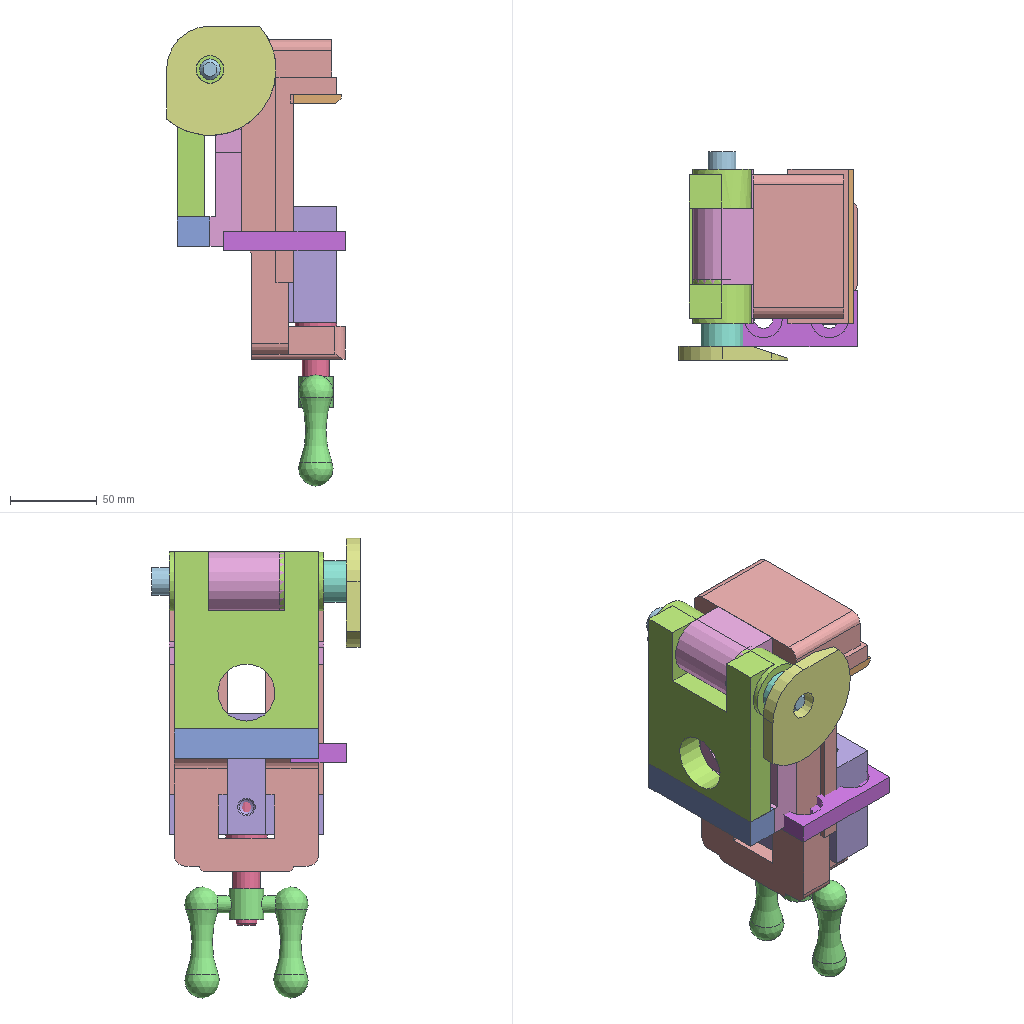Assembly | NX | 11 different items | 11 placed | box 103 x 120 x 265 mm
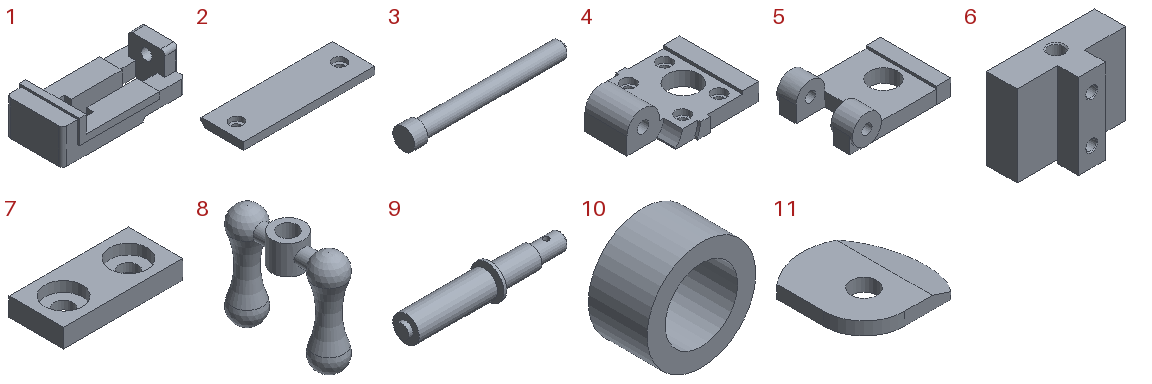Parts list (item | quantity | size | volume | features):
1 | x1 | 184 x 89 x 60 mm | 417123 mm3 | features DATUM_CSYS 9, EXTRUDE 8, SKETCH 8, SIMPLE HOLE 6, SYMBOLIC_THREAD 6, HOLE PACKAGE 3, BLEND 1, CBORE_HOLE 1
2 | x1 | 89 x 29 x 5 mm | 12044 mm3 | features DATUM_CSYS 3, EXTRUDE 3, SKETCH 2
3 | x1 | 117 x 16 x 16 mm | 14045 mm3 | features DATUM_CSYS 2, CHAMFER 1, SKETCH 1, SWP104 1, SYMBOLIC_THREAD 1
4 | x1 | 119 x 89 x 35 mm | 132113 mm3 | features EXTRUDE 11, CBORE_HOLE 4, DATUM_CSYS 4, SKETCH 3, HOLE PACKAGE 1
5 | x1 | 119 x 89 x 36 mm | 149069 mm3 | features EXTRUDE 8, DATUM_CSYS 4, SKETCH 3, UNITE 3
6 | x1 | 89 x 42 x 70 mm | 164920 mm3 | features DATUM_CSYS 6, SIMPLE HOLE 5, SKETCH 5, SYMBOLIC_THREAD 5, HOLE PACKAGE 4, EXTRUDE 2
7 | x1 | 70 x 32 x 11 mm | 19128 mm3 | features DATUM_CSYS 2, EXTRUDE 2, SKETCH 1
8 | x1 | 20 x 71 x 64 mm | 28763 mm3 | features DATUM_CSYS 4, EXTRUDE 3, SKETCH 3, SWP104 2, UNITE 1
9 | x1 | 113 x 24 x 24 mm | 24723 mm3 | features DATUM_CSYS 3, SKETCH 2, CHAMFER 1, EXTRUDE 1, SWP104 1
10 | x1 | 24 x 13 x 24 mm | 3267 mm3 | features DATUM_CSYS 2, SKETCH 1, SWP104 1
11 | x1 | 62.986 x 63 x 8 mm | 22550 mm3 | features DATUM_CSYS 3, EXTRUDE 2, SKETCH 2
Mates (type | each side: item.copy, entity, surface, feature):
Fix | 1.1 component
AlignLock | 2.1 face cylinder Extrude(3) | 1.1 face cylinder M4 x 0.7 Threaded Hole(13) | 2 times
Touch | 2.1 face plane Extrude(2) | 1.1 face plane Extrude(3)
Touch | 9.1 face plane Revolve(2) | 6.1 face plane Extrude(2)
AlignLock | 9.1 face cylinder Revolve(2) | 1.1 face cylinder Ø16 Counterbored Hole(17)
Touch | 1.1 face plane Extrude(6) | 9.1 face plane Revolve(2)
Touch | 6.1 face plane Extrude(3) | 1.1 face plane Extrude(4)
Touch | 6.1 face plane Extrude(2) | 1.1 face plane Extrude(4)
Touch | 4.1 face plane Extrude(4) | 5.1 face plane Extrude(4)
AlignLock | 4.1 face cylinder Extrude(13) | 5.1 face cylinder Extrude(8)
Touch | 4.1 face plane Extrude(3) | 5.1 face plane Extrude(4)
AlignLock | 4.1 face cylinder Ø10 Counterbored Hole(14) | 1.1 face cylinder M8 x 1.25 Threaded Hole(14) | 2 times
AlignLock | 1.1 face cylinder M8 x 1.25 Threaded Hole(14) | 4.1 face cylinder Ø10 Counterbored Hole(14)
Touch | 1.1 face plane Extrude(2) | 4.1 face plane Extrude(2)
AlignLock | 8.1 face cylinder Extrude(2) | 9.1 face cylinder Revolve(2)
Touch | 8.1 face plane Extrude(2) | 9.1 face plane Revolve(2)
AlignLock | 3.1 face cylinder Revolve(2) | 5.1 face cylinder Extrude(8)
Touch | 3.1 face plane Revolve(2) | 5.1 face plane Extrude(12)
AlignLock | 10.1 face cylinder Revolve(2) | 3.1 face cylinder Revolve(2)
Touch | 5.1 face plane Extrude(8) | 10.1 face plane Revolve(2)
Touch | 11.1 face cylinder Extrude(2) | 3.1 face cylinder Revolve(2)
Touch | 11.1 face plane Extrude(2) | 10.1 face plane Revolve(2)
Parallel | 11.1 face plane Extrude(2) | 5.1 face plane Extrude(2)